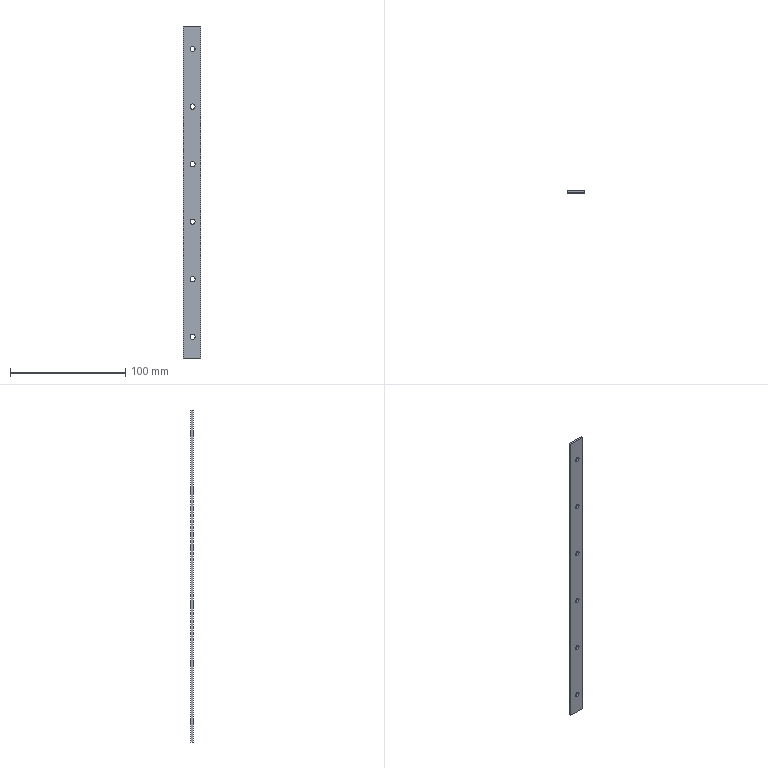Part | STEP file | Strip (L) | 1 solid | 18 faces | box 15 x 2 x 288.5 mm | volume 8464 mm3 | cylinder 12 | plane 6 | commonest cylinder face diameters 4.5 x12
STEP:
#1=CARTESIAN_POINT('',(0.,0.,0.));
#2=DIRECTION('',(0.,0.,1.));
#3=DIRECTION('',(1.,0.,0.));
#4=AXIS2_PLACEMENT_3D('',#1,#2,#3);
#5=CARTESIAN_POINT('',(8.,0.,16.25));
#6=VERTEX_POINT('',#5);
#7=CARTESIAN_POINT('',(8.,-2.,16.25));
#8=VERTEX_POINT('',#7);
#9=CARTESIAN_POINT('',(8.,-2.,16.25));
#10=DIRECTION('',(0.,-1.,0.));
#11=VECTOR('',#10,1.);
#12=LINE('',#9,#11);
#13=CARTESIAN_POINT('',(8.,-2.,18.5));
#14=DIRECTION('',(0.,-1.,0.));
#15=DIRECTION('',(0.,0.,-1.));
#16=AXIS2_PLACEMENT_3D('',#13,#14,#15);
#17=CYLINDRICAL_SURFACE('',#16,2.25);
#18=CARTESIAN_POINT('',(6.283,0.));
#19=DIRECTION('',(0.,1.));
#20=VECTOR('',#19,1.);
#21=LINE('',#18,#20);
#22=(GEOMETRIC_REPRESENTATION_CONTEXT(2)PARAMETRIC_REPRESENTATION_CONTEXT()REPRESENTATION_CONTEXT('',''));
#23=DEFINITIONAL_REPRESENTATION('',(#21),#22);
#24=PCURVE('',#17,#23);
#25=CARTESIAN_POINT('',(8.,-2.,18.5));
#26=DIRECTION('',(0.,-1.,0.));
#27=DIRECTION('',(0.,0.,-1.));
#28=AXIS2_PLACEMENT_3D('',#25,#26,#27);
#29=CYLINDRICAL_SURFACE('',#28,2.25);
#30=CARTESIAN_POINT('',(0.,0.));
#31=DIRECTION('',(0.,1.));
#32=VECTOR('',#31,1.);
#33=LINE('',#30,#32);
#34=(GEOMETRIC_REPRESENTATION_CONTEXT(2)PARAMETRIC_REPRESENTATION_CONTEXT()REPRESENTATION_CONTEXT('',''));
#35=DEFINITIONAL_REPRESENTATION('',(#33),#34);
#36=PCURVE('',#29,#35);
#37=SURFACE_CURVE('',#12,(#24,#36),.PCURVE_S1.);
#38=EDGE_CURVE('',#6,#8,#37,.T.);
#39=ORIENTED_EDGE('',*,*,#38,.T.);
#40=CARTESIAN_POINT('',(8.,-2.,20.75));
#41=VERTEX_POINT('',#40);
#42=CARTESIAN_POINT('',(8.,-2.,18.5));
#43=DIRECTION('',(0.,-1.,0.));
#44=DIRECTION('',(0.,0.,-1.));
#45=AXIS2_PLACEMENT_3D('',#42,#43,#44);
#46=CIRCLE('',#45,2.25);
#47=CARTESIAN_POINT('',(0.,0.));
#48=DIRECTION('',(1.,0.));
#49=VECTOR('',#48,1.);
#50=LINE('',#47,#49);
#51=(GEOMETRIC_REPRESENTATION_CONTEXT(2)PARAMETRIC_REPRESENTATION_CONTEXT()REPRESENTATION_CONTEXT('',''));
#52=DEFINITIONAL_REPRESENTATION('',(#50),#51);
#53=PCURVE('',#17,#52);
#54=CARTESIAN_POINT('',(0.,-2.,288.5));
#55=DIRECTION('',(0.,1.,0.));
#56=DIRECTION('',(0.,0.,1.));
#57=AXIS2_PLACEMENT_3D('',#54,#55,#56);
#58=PLANE('',#57);
#59=CARTESIAN_POINT('',(-272.25,8.));
#60=CARTESIAN_POINT('',(-272.25,11.897));
#61=CARTESIAN_POINT('',(-268.875,9.949));
#62=CARTESIAN_POINT('',(-265.5,8.));
#63=CARTESIAN_POINT('',(-268.875,6.051));
#64=CARTESIAN_POINT('',(-272.25,4.103));
#65=CARTESIAN_POINT('',(-272.25,8.));
#66=(BOUNDED_CURVE()B_SPLINE_CURVE(2,(#59,#60,#61,#62,#63,#64,#65),.UNSPECIFIED.,.T.,.F.)B_SPLINE_CURVE_WITH_KNOTS((1,2,2,2,2,1),(-2.094,0.,2.094,4.189,6.283,8.378),.UNSPECIFIED.)CURVE()GEOMETRIC_REPRESENTATION_ITEM()RATIONAL_B_SPLINE_CURVE((1.,0.5,1.,0.5,1.,0.5,1.))REPRESENTATION_ITEM(''));
#67=(GEOMETRIC_REPRESENTATION_CONTEXT(2)PARAMETRIC_REPRESENTATION_CONTEXT()REPRESENTATION_CONTEXT('',''));
#68=DEFINITIONAL_REPRESENTATION('',(#66),#67);
#69=PCURVE('',#58,#68);
#70=SURFACE_CURVE('',#46,(#53,#69),.PCURVE_S1.);
#71=EDGE_CURVE('',#41,#8,#70,.T.);
#72=ORIENTED_EDGE('',*,*,#71,.F.);
#73=CARTESIAN_POINT('',(8.,0.,20.75));
#74=VERTEX_POINT('',#73);
#75=CARTESIAN_POINT('',(8.,-2.,20.75));
#76=DIRECTION('',(0.,-1.,0.));
#77=VECTOR('',#76,1.);
#78=LINE('',#75,#77);
#79=CARTESIAN_POINT('',(3.142,0.));
#80=DIRECTION('',(0.,1.));
#81=VECTOR('',#80,1.);
#82=LINE('',#79,#81);
#83=(GEOMETRIC_REPRESENTATION_CONTEXT(2)PARAMETRIC_REPRESENTATION_CONTEXT()REPRESENTATION_CONTEXT('',''));
#84=DEFINITIONAL_REPRESENTATION('',(#82),#83);
#85=PCURVE('',#17,#84);
#86=CARTESIAN_POINT('',(3.142,0.));
#87=DIRECTION('',(0.,1.));
#88=VECTOR('',#87,1.);
#89=LINE('',#86,#88);
#90=(GEOMETRIC_REPRESENTATION_CONTEXT(2)PARAMETRIC_REPRESENTATION_CONTEXT()REPRESENTATION_CONTEXT('',''));
#91=DEFINITIONAL_REPRESENTATION('',(#89),#90);
#92=PCURVE('',#29,#91);
#93=SURFACE_CURVE('',#78,(#85,#92),.PCURVE_S1.);
#94=EDGE_CURVE('',#74,#41,#93,.T.);
#95=ORIENTED_EDGE('',*,*,#94,.F.);
#96=CARTESIAN_POINT('',(8.,0.,18.5));
#97=DIRECTION('',(0.,-1.,0.));
#98=DIRECTION('',(0.,0.,-1.));
#99=AXIS2_PLACEMENT_3D('',#96,#97,#98);
#100=CIRCLE('',#99,2.25);
#101=CARTESIAN_POINT('',(0.,-2.));
#102=DIRECTION('',(1.,0.));
#103=VECTOR('',#102,1.);
#104=LINE('',#101,#103);
#105=(GEOMETRIC_REPRESENTATION_CONTEXT(2)PARAMETRIC_REPRESENTATION_CONTEXT()REPRESENTATION_CONTEXT('',''));
#106=DEFINITIONAL_REPRESENTATION('',(#104),#105);
#107=PCURVE('',#17,#106);
#108=CARTESIAN_POINT('',(0.,0.,288.5));
#109=DIRECTION('',(0.,-1.,0.));
#110=DIRECTION('',(0.,0.,-1.));
#111=AXIS2_PLACEMENT_3D('',#108,#109,#110);
#112=PLANE('',#111);
#113=CARTESIAN_POINT('',(270.,8.));
#114=DIRECTION('',(1.,0.));
#115=AXIS2_PLACEMENT_2D('',#113,#114);
#116=CIRCLE('',#115,2.25);
#117=(GEOMETRIC_REPRESENTATION_CONTEXT(2)PARAMETRIC_REPRESENTATION_CONTEXT()REPRESENTATION_CONTEXT('',''));
#118=DEFINITIONAL_REPRESENTATION('',(#116),#117);
#119=PCURVE('',#112,#118);
#120=SURFACE_CURVE('',#100,(#107,#119),.PCURVE_S1.);
#121=EDGE_CURVE('',#74,#6,#120,.T.);
#122=ORIENTED_EDGE('',*,*,#121,.T.);
#123=EDGE_LOOP('',(#39,#72,#95,#122));
#124=FACE_BOUND('',#123,.F.);
#125=ADVANCED_FACE('',(#124),#17,.F.);
#126=CARTESIAN_POINT('',(8.,0.,66.25));
#127=VERTEX_POINT('',#126);
#128=CARTESIAN_POINT('',(8.,-2.,66.25));
#129=VERTEX_POINT('',#128);
#130=CARTESIAN_POINT('',(8.,-2.,66.25));
#131=DIRECTION('',(0.,-1.,0.));
#132=VECTOR('',#131,1.);
#133=LINE('',#130,#132);
#134=CARTESIAN_POINT('',(8.,-2.,68.5));
#135=DIRECTION('',(0.,-1.,0.));
#136=DIRECTION('',(0.,0.,-1.));
#137=AXIS2_PLACEMENT_3D('',#134,#135,#136);
#138=CYLINDRICAL_SURFACE('',#137,2.25);
#139=CARTESIAN_POINT('',(6.283,0.));
#140=DIRECTION('',(0.,1.));
#141=VECTOR('',#140,1.);
#142=LINE('',#139,#141);
#143=(GEOMETRIC_REPRESENTATION_CONTEXT(2)PARAMETRIC_REPRESENTATION_CONTEXT()REPRESENTATION_CONTEXT('',''));
#144=DEFINITIONAL_REPRESENTATION('',(#142),#143);
#145=PCURVE('',#138,#144);
#146=CARTESIAN_POINT('',(8.,-2.,68.5));
#147=DIRECTION('',(0.,-1.,0.));
#148=DIRECTION('',(0.,0.,-1.));
#149=AXIS2_PLACEMENT_3D('',#146,#147,#148);
#150=CYLINDRICAL_SURFACE('',#149,2.25);
#151=CARTESIAN_POINT('',(0.,0.));
#152=DIRECTION('',(0.,1.));
#153=VECTOR('',#152,1.);
#154=LINE('',#151,#153);
#155=(GEOMETRIC_REPRESENTATION_CONTEXT(2)PARAMETRIC_REPRESENTATION_CONTEXT()REPRESENTATION_CONTEXT('',''));
#156=DEFINITIONAL_REPRESENTATION('',(#154),#155);
#157=PCURVE('',#150,#156);
#158=SURFACE_CURVE('',#133,(#145,#157),.PCURVE_S1.);
#159=EDGE_CURVE('',#127,#129,#158,.T.);
#160=ORIENTED_EDGE('',*,*,#159,.T.);
#161=CARTESIAN_POINT('',(8.,-2.,70.75));
#162=VERTEX_POINT('',#161);
#163=CARTESIAN_POINT('',(8.,-2.,68.5));
#164=DIRECTION('',(0.,-1.,0.));
#165=DIRECTION('',(0.,0.,-1.));
#166=AXIS2_PLACEMENT_3D('',#163,#164,#165);
#167=CIRCLE('',#166,2.25);
#168=CARTESIAN_POINT('',(0.,0.));
#169=DIRECTION('',(1.,0.));
#170=VECTOR('',#169,1.);
#171=LINE('',#168,#170);
#172=(GEOMETRIC_REPRESENTATION_CONTEXT(2)PARAMETRIC_REPRESENTATION_CONTEXT()REPRESENTATION_CONTEXT('',''));
#173=DEFINITIONAL_REPRESENTATION('',(#171),#172);
#174=PCURVE('',#138,#173);
#175=CARTESIAN_POINT('',(-222.25,8.));
#176=CARTESIAN_POINT('',(-222.25,11.897));
#177=CARTESIAN_POINT('',(-218.875,9.949));
#178=CARTESIAN_POINT('',(-215.5,8.));
#179=CARTESIAN_POINT('',(-218.875,6.051));
#180=CARTESIAN_POINT('',(-222.25,4.103));
#181=CARTESIAN_POINT('',(-222.25,8.));
#182=(BOUNDED_CURVE()B_SPLINE_CURVE(2,(#175,#176,#177,#178,#179,#180,#181),.UNSPECIFIED.,.T.,.F.)B_SPLINE_CURVE_WITH_KNOTS((1,2,2,2,2,1),(-2.094,0.,2.094,4.189,6.283,8.378),.UNSPECIFIED.)CURVE()GEOMETRIC_REPRESENTATION_ITEM()RATIONAL_B_SPLINE_CURVE((1.,0.5,1.,0.5,1.,0.5,1.))REPRESENTATION_ITEM(''));
#183=(GEOMETRIC_REPRESENTATION_CONTEXT(2)PARAMETRIC_REPRESENTATION_CONTEXT()REPRESENTATION_CONTEXT('',''));
#184=DEFINITIONAL_REPRESENTATION('',(#182),#183);
#185=PCURVE('',#58,#184);
#186=SURFACE_CURVE('',#167,(#174,#185),.PCURVE_S1.);
#187=EDGE_CURVE('',#162,#129,#186,.T.);
#188=ORIENTED_EDGE('',*,*,#187,.F.);
#189=CARTESIAN_POINT('',(8.,0.,70.75));
#190=VERTEX_POINT('',#189);
#191=CARTESIAN_POINT('',(8.,-2.,70.75));
#192=DIRECTION('',(0.,-1.,0.));
#193=VECTOR('',#192,1.);
#194=LINE('',#191,#193);
#195=CARTESIAN_POINT('',(3.142,0.));
#196=DIRECTION('',(0.,1.));
#197=VECTOR('',#196,1.);
#198=LINE('',#195,#197);
#199=(GEOMETRIC_REPRESENTATION_CONTEXT(2)PARAMETRIC_REPRESENTATION_CONTEXT()REPRESENTATION_CONTEXT('',''));
#200=DEFINITIONAL_REPRESENTATION('',(#198),#199);
#201=PCURVE('',#138,#200);
#202=CARTESIAN_POINT('',(3.142,0.));
#203=DIRECTION('',(0.,1.));
#204=VECTOR('',#203,1.);
#205=LINE('',#202,#204);
#206=(GEOMETRIC_REPRESENTATION_CONTEXT(2)PARAMETRIC_REPRESENTATION_CONTEXT()REPRESENTATION_CONTEXT('',''));
#207=DEFINITIONAL_REPRESENTATION('',(#205),#206);
#208=PCURVE('',#150,#207);
#209=SURFACE_CURVE('',#194,(#201,#208),.PCURVE_S1.);
#210=EDGE_CURVE('',#190,#162,#209,.T.);
#211=ORIENTED_EDGE('',*,*,#210,.F.);
#212=CARTESIAN_POINT('',(8.,0.,68.5));
#213=DIRECTION('',(0.,-1.,0.));
#214=DIRECTION('',(0.,0.,-1.));
#215=AXIS2_PLACEMENT_3D('',#212,#213,#214);
#216=CIRCLE('',#215,2.25);
#217=CARTESIAN_POINT('',(0.,-2.));
#218=DIRECTION('',(1.,0.));
#219=VECTOR('',#218,1.);
#220=LINE('',#217,#219);
#221=(GEOMETRIC_REPRESENTATION_CONTEXT(2)PARAMETRIC_REPRESENTATION_CONTEXT()REPRESENTATION_CONTEXT('',''));
#222=DEFINITIONAL_REPRESENTATION('',(#220),#221);
#223=PCURVE('',#138,#222);
#224=CARTESIAN_POINT('',(220.,8.));
#225=DIRECTION('',(1.,0.));
#226=AXIS2_PLACEMENT_2D('',#224,#225);
#227=CIRCLE('',#226,2.25);
#228=(GEOMETRIC_REPRESENTATION_CONTEXT(2)PARAMETRIC_REPRESENTATION_CONTEXT()REPRESENTATION_CONTEXT('',''));
#229=DEFINITIONAL_REPRESENTATION('',(#227),#228);
#230=PCURVE('',#112,#229);
#231=SURFACE_CURVE('',#216,(#223,#230),.PCURVE_S1.);
#232=EDGE_CURVE('',#190,#127,#231,.T.);
#233=ORIENTED_EDGE('',*,*,#232,.T.);
#234=EDGE_LOOP('',(#160,#188,#211,#233));
#235=FACE_BOUND('',#234,.F.);
#236=ADVANCED_FACE('',(#235),#138,.F.);
#237=CARTESIAN_POINT('',(8.,0.,116.25));
#238=VERTEX_POINT('',#237);
#239=CARTESIAN_POINT('',(8.,-2.,116.25));
#240=VERTEX_POINT('',#239);
#241=CARTESIAN_POINT('',(8.,-2.,116.25));
#242=DIRECTION('',(0.,-1.,0.));
#243=VECTOR('',#242,1.);
#244=LINE('',#241,#243);
#245=CARTESIAN_POINT('',(8.,-2.,118.5));
#246=DIRECTION('',(0.,-1.,0.));
#247=DIRECTION('',(0.,0.,-1.));
#248=AXIS2_PLACEMENT_3D('',#245,#246,#247);
#249=CYLINDRICAL_SURFACE('',#248,2.25);
#250=CARTESIAN_POINT('',(6.283,0.));
#251=DIRECTION('',(0.,1.));
#252=VECTOR('',#251,1.);
#253=LINE('',#250,#252);
#254=(GEOMETRIC_REPRESENTATION_CONTEXT(2)PARAMETRIC_REPRESENTATION_CONTEXT()REPRESENTATION_CONTEXT('',''));
#255=DEFINITIONAL_REPRESENTATION('',(#253),#254);
#256=PCURVE('',#249,#255);
#257=CARTESIAN_POINT('',(8.,-2.,118.5));
#258=DIRECTION('',(0.,-1.,0.));
#259=DIRECTION('',(0.,0.,-1.));
#260=AXIS2_PLACEMENT_3D('',#257,#258,#259);
#261=CYLINDRICAL_SURFACE('',#260,2.25);
#262=CARTESIAN_POINT('',(0.,0.));
#263=DIRECTION('',(0.,1.));
#264=VECTOR('',#263,1.);
#265=LINE('',#262,#264);
#266=(GEOMETRIC_REPRESENTATION_CONTEXT(2)PARAMETRIC_REPRESENTATION_CONTEXT()REPRESENTATION_CONTEXT('',''));
#267=DEFINITIONAL_REPRESENTATION('',(#265),#266);
#268=PCURVE('',#261,#267);
#269=SURFACE_CURVE('',#244,(#256,#268),.PCURVE_S1.);
#270=EDGE_CURVE('',#238,#240,#269,.T.);
#271=ORIENTED_EDGE('',*,*,#270,.T.);
#272=CARTESIAN_POINT('',(8.,-2.,120.75));
#273=VERTEX_POINT('',#272);
#274=CARTESIAN_POINT('',(8.,-2.,118.5));
#275=DIRECTION('',(0.,-1.,0.));
#276=DIRECTION('',(0.,0.,-1.));
#277=AXIS2_PLACEMENT_3D('',#274,#275,#276);
#278=CIRCLE('',#277,2.25);
#279=CARTESIAN_POINT('',(0.,0.));
#280=DIRECTION('',(1.,0.));
#281=VECTOR('',#280,1.);
#282=LINE('',#279,#281);
#283=(GEOMETRIC_REPRESENTATION_CONTEXT(2)PARAMETRIC_REPRESENTATION_CONTEXT()REPRESENTATION_CONTEXT('',''));
#284=DEFINITIONAL_REPRESENTATION('',(#282),#283);
#285=PCURVE('',#249,#284);
#286=CARTESIAN_POINT('',(-172.25,8.));
#287=CARTESIAN_POINT('',(-172.25,11.897));
#288=CARTESIAN_POINT('',(-168.875,9.949));
#289=CARTESIAN_POINT('',(-165.5,8.));
#290=CARTESIAN_POINT('',(-168.875,6.051));
#291=CARTESIAN_POINT('',(-172.25,4.103));
#292=CARTESIAN_POINT('',(-172.25,8.));
#293=(BOUNDED_CURVE()B_SPLINE_CURVE(2,(#286,#287,#288,#289,#290,#291,#292),.UNSPECIFIED.,.T.,.F.)B_SPLINE_CURVE_WITH_KNOTS((1,2,2,2,2,1),(-2.094,0.,2.094,4.189,6.283,8.378),.UNSPECIFIED.)CURVE()GEOMETRIC_REPRESENTATION_ITEM()RATIONAL_B_SPLINE_CURVE((1.,0.5,1.,0.5,1.,0.5,1.))REPRESENTATION_ITEM(''));
#294=(GEOMETRIC_REPRESENTATION_CONTEXT(2)PARAMETRIC_REPRESENTATION_CONTEXT()REPRESENTATION_CONTEXT('',''));
#295=DEFINITIONAL_REPRESENTATION('',(#293),#294);
#296=PCURVE('',#58,#295);
#297=SURFACE_CURVE('',#278,(#285,#296),.PCURVE_S1.);
#298=EDGE_CURVE('',#273,#240,#297,.T.);
#299=ORIENTED_EDGE('',*,*,#298,.F.);
#300=CARTESIAN_POINT('',(8.,0.,120.75));
#301=VERTEX_POINT('',#300);
#302=CARTESIAN_POINT('',(8.,-2.,120.75));
#303=DIRECTION('',(0.,-1.,0.));
#304=VECTOR('',#303,1.);
#305=LINE('',#302,#304);
#306=CARTESIAN_POINT('',(3.142,0.));
#307=DIRECTION('',(0.,1.));
#308=VECTOR('',#307,1.);
#309=LINE('',#306,#308);
#310=(GEOMETRIC_REPRESENTATION_CONTEXT(2)PARAMETRIC_REPRESENTATION_CONTEXT()REPRESENTATION_CONTEXT('',''));
#311=DEFINITIONAL_REPRESENTATION('',(#309),#310);
#312=PCURVE('',#249,#311);
#313=CARTESIAN_POINT('',(3.142,0.));
#314=DIRECTION('',(0.,1.));
#315=VECTOR('',#314,1.);
#316=LINE('',#313,#315);
#317=(GEOMETRIC_REPRESENTATION_CONTEXT(2)PARAMETRIC_REPRESENTATION_CONTEXT()REPRESENTATION_CONTEXT('',''));
#318=DEFINITIONAL_REPRESENTATION('',(#316),#317);
#319=PCURVE('',#261,#318);
#320=SURFACE_CURVE('',#305,(#312,#319),.PCURVE_S1.);
#321=EDGE_CURVE('',#301,#273,#320,.T.);
#322=ORIENTED_EDGE('',*,*,#321,.F.);
#323=CARTESIAN_POINT('',(8.,0.,118.5));
#324=DIRECTION('',(0.,-1.,0.));
#325=DIRECTION('',(0.,0.,-1.));
#326=AXIS2_PLACEMENT_3D('',#323,#324,#325);
#327=CIRCLE('',#326,2.25);
#328=CARTESIAN_POINT('',(0.,-2.));
#329=DIRECTION('',(1.,0.));
#330=VECTOR('',#329,1.);
#331=LINE('',#328,#330);
#332=(GEOMETRIC_REPRESENTATION_CONTEXT(2)PARAMETRIC_REPRESENTATION_CONTEXT()REPRESENTATION_CONTEXT('',''));
#333=DEFINITIONAL_REPRESENTATION('',(#331),#332);
#334=PCURVE('',#249,#333);
#335=CARTESIAN_POINT('',(170.,8.));
#336=DIRECTION('',(1.,0.));
#337=AXIS2_PLACEMENT_2D('',#335,#336);
#338=CIRCLE('',#337,2.25);
#339=(GEOMETRIC_REPRESENTATION_CONTEXT(2)PARAMETRIC_REPRESENTATION_CONTEXT()REPRESENTATION_CONTEXT('',''));
#340=DEFINITIONAL_REPRESENTATION('',(#338),#339);
#341=PCURVE('',#112,#340);
#342=SURFACE_CURVE('',#327,(#334,#341),.PCURVE_S1.);
#343=EDGE_CURVE('',#301,#238,#342,.T.);
#344=ORIENTED_EDGE('',*,*,#343,.T.);
#345=EDGE_LOOP('',(#271,#299,#322,#344));
#346=FACE_BOUND('',#345,.F.);
#347=ADVANCED_FACE('',(#346),#249,.F.);
#348=CARTESIAN_POINT('',(8.,0.,166.25));
#349=VERTEX_POINT('',#348);
#350=CARTESIAN_POINT('',(8.,-2.,166.25));
#351=VERTEX_POINT('',#350);
#352=CARTESIAN_POINT('',(8.,-2.,166.25));
#353=DIRECTION('',(0.,-1.,0.));
#354=VECTOR('',#353,1.);
#355=LINE('',#352,#354);
#356=CARTESIAN_POINT('',(8.,-2.,168.5));
#357=DIRECTION('',(0.,-1.,0.));
#358=DIRECTION('',(0.,0.,-1.));
#359=AXIS2_PLACEMENT_3D('',#356,#357,#358);
#360=CYLINDRICAL_SURFACE('',#359,2.25);
#361=CARTESIAN_POINT('',(6.283,0.));
#362=DIRECTION('',(0.,1.));
#363=VECTOR('',#362,1.);
#364=LINE('',#361,#363);
#365=(GEOMETRIC_REPRESENTATION_CONTEXT(2)PARAMETRIC_REPRESENTATION_CONTEXT()REPRESENTATION_CONTEXT('',''));
#366=DEFINITIONAL_REPRESENTATION('',(#364),#365);
#367=PCURVE('',#360,#366);
#368=CARTESIAN_POINT('',(8.,-2.,168.5));
#369=DIRECTION('',(0.,-1.,0.));
#370=DIRECTION('',(0.,0.,-1.));
#371=AXIS2_PLACEMENT_3D('',#368,#369,#370);
#372=CYLINDRICAL_SURFACE('',#371,2.25);
#373=CARTESIAN_POINT('',(0.,0.));
#374=DIRECTION('',(0.,1.));
#375=VECTOR('',#374,1.);
#376=LINE('',#373,#375);
#377=(GEOMETRIC_REPRESENTATION_CONTEXT(2)PARAMETRIC_REPRESENTATION_CONTEXT()REPRESENTATION_CONTEXT('',''));
#378=DEFINITIONAL_REPRESENTATION('',(#376),#377);
#379=PCURVE('',#372,#378);
#380=SURFACE_CURVE('',#355,(#367,#379),.PCURVE_S1.);
#381=EDGE_CURVE('',#349,#351,#380,.T.);
#382=ORIENTED_EDGE('',*,*,#381,.T.);
#383=CARTESIAN_POINT('',(8.,-2.,170.75));
#384=VERTEX_POINT('',#383);
#385=CARTESIAN_POINT('',(8.,-2.,168.5));
#386=DIRECTION('',(0.,-1.,0.));
#387=DIRECTION('',(0.,0.,-1.));
#388=AXIS2_PLACEMENT_3D('',#385,#386,#387);
#389=CIRCLE('',#388,2.25);
#390=CARTESIAN_POINT('',(0.,0.));
#391=DIRECTION('',(1.,0.));
#392=VECTOR('',#391,1.);
#393=LINE('',#390,#392);
#394=(GEOMETRIC_REPRESENTATION_CONTEXT(2)PARAMETRIC_REPRESENTATION_CONTEXT()REPRESENTATION_CONTEXT('',''));
#395=DEFINITIONAL_REPRESENTATION('',(#393),#394);
#396=PCURVE('',#360,#395);
#397=CARTESIAN_POINT('',(-122.25,8.));
#398=CARTESIAN_POINT('',(-122.25,11.897));
#399=CARTESIAN_POINT('',(-118.875,9.949));
#400=CARTESIAN_POINT('',(-115.5,8.));
#401=CARTESIAN_POINT('',(-118.875,6.051));
#402=CARTESIAN_POINT('',(-122.25,4.103));
#403=CARTESIAN_POINT('',(-122.25,8.));
#404=(BOUNDED_CURVE()B_SPLINE_CURVE(2,(#397,#398,#399,#400,#401,#402,#403),.UNSPECIFIED.,.T.,.F.)B_SPLINE_CURVE_WITH_KNOTS((1,2,2,2,2,1),(-2.094,0.,2.094,4.189,6.283,8.378),.UNSPECIFIED.)CURVE()GEOMETRIC_REPRESENTATION_ITEM()RATIONAL_B_SPLINE_CURVE((1.,0.5,1.,0.5,1.,0.5,1.))REPRESENTATION_ITEM(''));
#405=(GEOMETRIC_REPRESENTATION_CONTEXT(2)PARAMETRIC_REPRESENTATION_CONTEXT()REPRESENTATION_CONTEXT('',''));
#406=DEFINITIONAL_REPRESENTATION('',(#404),#405);
#407=PCURVE('',#58,#406);
#408=SURFACE_CURVE('',#389,(#396,#407),.PCURVE_S1.);
#409=EDGE_CURVE('',#384,#351,#408,.T.);
#410=ORIENTED_EDGE('',*,*,#409,.F.);
#411=CARTESIAN_POINT('',(8.,0.,170.75));
#412=VERTEX_POINT('',#411);
#413=CARTESIAN_POINT('',(8.,-2.,170.75));
#414=DIRECTION('',(0.,-1.,0.));
#415=VECTOR('',#414,1.);
#416=LINE('',#413,#415);
#417=CARTESIAN_POINT('',(3.142,0.));
#418=DIRECTION('',(0.,1.));
#419=VECTOR('',#418,1.);
#420=LINE('',#417,#419);
#421=(GEOMETRIC_REPRESENTATION_CONTEXT(2)PARAMETRIC_REPRESENTATION_CONTEXT()REPRESENTATION_CONTEXT('',''));
#422=DEFINITIONAL_REPRESENTATION('',(#420),#421);
#423=PCURVE('',#360,#422);
#424=CARTESIAN_POINT('',(3.142,0.));
#425=DIRECTION('',(0.,1.));
#426=VECTOR('',#425,1.);
#427=LINE('',#424,#426);
#428=(GEOMETRIC_REPRESENTATION_CONTEXT(2)PARAMETRIC_REPRESENTATION_CONTEXT()REPRESENTATION_CONTEXT('',''));
#429=DEFINITIONAL_REPRESENTATION('',(#427),#428);
#430=PCURVE('',#372,#429);
#431=SURFACE_CURVE('',#416,(#423,#430),.PCURVE_S1.);
#432=EDGE_CURVE('',#412,#384,#431,.T.);
#433=ORIENTED_EDGE('',*,*,#432,.F.);
#434=CARTESIAN_POINT('',(8.,0.,168.5));
#435=DIRECTION('',(0.,-1.,0.));
#436=DIRECTION('',(0.,0.,-1.));
#437=AXIS2_PLACEMENT_3D('',#434,#435,#436);
#438=CIRCLE('',#437,2.25);
#439=CARTESIAN_POINT('',(0.,-2.));
#440=DIRECTION('',(1.,0.));
#441=VECTOR('',#440,1.);
#442=LINE('',#439,#441);
#443=(GEOMETRIC_REPRESENTATION_CONTEXT(2)PARAMETRIC_REPRESENTATION_CONTEXT()REPRESENTATION_CONTEXT('',''));
#444=DEFINITIONAL_REPRESENTATION('',(#442),#443);
#445=PCURVE('',#360,#444);
#446=CARTESIAN_POINT('',(120.,8.));
#447=DIRECTION('',(1.,0.));
#448=AXIS2_PLACEMENT_2D('',#446,#447);
#449=CIRCLE('',#448,2.25);
#450=(GEOMETRIC_REPRESENTATION_CONTEXT(2)PARAMETRIC_REPRESENTATION_CONTEXT()REPRESENTATION_CONTEXT('',''));
#451=DEFINITIONAL_REPRESENTATION('',(#449),#450);
#452=PCURVE('',#112,#451);
#453=SURFACE_CURVE('',#438,(#445,#452),.PCURVE_S1.);
#454=EDGE_CURVE('',#412,#349,#453,.T.);
#455=ORIENTED_EDGE('',*,*,#454,.T.);
#456=EDGE_LOOP('',(#382,#410,#433,#455));
#457=FACE_BOUND('',#456,.F.);
#458=ADVANCED_FACE('',(#457),#360,.F.);
#459=CARTESIAN_POINT('',(8.,0.,216.25));
#460=VERTEX_POINT('',#459);
#461=CARTESIAN_POINT('',(8.,-2.,216.25));
#462=VERTEX_POINT('',#461);
#463=CARTESIAN_POINT('',(8.,-2.,216.25));
#464=DIRECTION('',(0.,-1.,0.));
#465=VECTOR('',#464,1.);
#466=LINE('',#463,#465);
#467=CARTESIAN_POINT('',(8.,-2.,218.5));
#468=DIRECTION('',(0.,-1.,0.));
#469=DIRECTION('',(0.,0.,-1.));
#470=AXIS2_PLACEMENT_3D('',#467,#468,#469);
#471=CYLINDRICAL_SURFACE('',#470,2.25);
#472=CARTESIAN_POINT('',(6.283,0.));
#473=DIRECTION('',(0.,1.));
#474=VECTOR('',#473,1.);
#475=LINE('',#472,#474);
#476=(GEOMETRIC_REPRESENTATION_CONTEXT(2)PARAMETRIC_REPRESENTATION_CONTEXT()REPRESENTATION_CONTEXT('',''));
#477=DEFINITIONAL_REPRESENTATION('',(#475),#476);
#478=PCURVE('',#471,#477);
#479=CARTESIAN_POINT('',(8.,-2.,218.5));
#480=DIRECTION('',(0.,-1.,0.));
#481=DIRECTION('',(0.,0.,-1.));
#482=AXIS2_PLACEMENT_3D('',#479,#480,#481);
#483=CYLINDRICAL_SURFACE('',#482,2.25);
#484=CARTESIAN_POINT('',(0.,0.));
#485=DIRECTION('',(0.,1.));
#486=VECTOR('',#485,1.);
#487=LINE('',#484,#486);
#488=(GEOMETRIC_REPRESENTATION_CONTEXT(2)PARAMETRIC_REPRESENTATION_CONTEXT()REPRESENTATION_CONTEXT('',''));
#489=DEFINITIONAL_REPRESENTATION('',(#487),#488);
#490=PCURVE('',#483,#489);
#491=SURFACE_CURVE('',#466,(#478,#490),.PCURVE_S1.);
#492=EDGE_CURVE('',#460,#462,#491,.T.);
#493=ORIENTED_EDGE('',*,*,#492,.T.);
#494=CARTESIAN_POINT('',(8.,-2.,220.75));
#495=VERTEX_POINT('',#494);
#496=CARTESIAN_POINT('',(8.,-2.,218.5));
#497=DIRECTION('',(0.,-1.,0.));
#498=DIRECTION('',(0.,0.,-1.));
#499=AXIS2_PLACEMENT_3D('',#496,#497,#498);
#500=CIRCLE('',#499,2.25);
#501=CARTESIAN_POINT('',(0.,0.));
#502=DIRECTION('',(1.,0.));
#503=VECTOR('',#502,1.);
#504=LINE('',#501,#503);
#505=(GEOMETRIC_REPRESENTATION_CONTEXT(2)PARAMETRIC_REPRESENTATION_CONTEXT()REPRESENTATION_CONTEXT('',''));
#506=DEFINITIONAL_REPRESENTATION('',(#504),#505);
#507=PCURVE('',#471,#506);
#508=CARTESIAN_POINT('',(-72.25,8.));
#509=CARTESIAN_POINT('',(-72.25,11.897));
#510=CARTESIAN_POINT('',(-68.875,9.949));
#511=CARTESIAN_POINT('',(-65.5,8.));
#512=CARTESIAN_POINT('',(-68.875,6.051));
#513=CARTESIAN_POINT('',(-72.25,4.103));
#514=CARTESIAN_POINT('',(-72.25,8.));
#515=(BOUNDED_CURVE()B_SPLINE_CURVE(2,(#508,#509,#510,#511,#512,#513,#514),.UNSPECIFIED.,.T.,.F.)B_SPLINE_CURVE_WITH_KNOTS((1,2,2,2,2,1),(-2.094,0.,2.094,4.189,6.283,8.378),.UNSPECIFIED.)CURVE()GEOMETRIC_REPRESENTATION_ITEM()RATIONAL_B_SPLINE_CURVE((1.,0.5,1.,0.5,1.,0.5,1.))REPRESENTATION_ITEM(''));
#516=(GEOMETRIC_REPRESENTATION_CONTEXT(2)PARAMETRIC_REPRESENTATION_CONTEXT()REPRESENTATION_CONTEXT('',''));
#517=DEFINITIONAL_REPRESENTATION('',(#515),#516);
#518=PCURVE('',#58,#517);
#519=SURFACE_CURVE('',#500,(#507,#518),.PCURVE_S1.);
#520=EDGE_CURVE('',#495,#462,#519,.T.);
#521=ORIENTED_EDGE('',*,*,#520,.F.);
#522=CARTESIAN_POINT('',(8.,0.,220.75));
#523=VERTEX_POINT('',#522);
#524=CARTESIAN_POINT('',(8.,-2.,220.75));
#525=DIRECTION('',(0.,-1.,0.));
#526=VECTOR('',#525,1.);
#527=LINE('',#524,#526);
#528=CARTESIAN_POINT('',(3.142,0.));
#529=DIRECTION('',(0.,1.));
#530=VECTOR('',#529,1.);
#531=LINE('',#528,#530);
#532=(GEOMETRIC_REPRESENTATION_CONTEXT(2)PARAMETRIC_REPRESENTATION_CONTEXT()REPRESENTATION_CONTEXT('',''));
#533=DEFINITIONAL_REPRESENTATION('',(#531),#532);
#534=PCURVE('',#471,#533);
#535=CARTESIAN_POINT('',(3.142,0.));
#536=DIRECTION('',(0.,1.));
#537=VECTOR('',#536,1.);
#538=LINE('',#535,#537);
#539=(GEOMETRIC_REPRESENTATION_CONTEXT(2)PARAMETRIC_REPRESENTATION_CONTEXT()REPRESENTATION_CONTEXT('',''));
#540=DEFINITIONAL_REPRESENTATION('',(#538),#539);
#541=PCURVE('',#483,#540);
#542=SURFACE_CURVE('',#527,(#534,#541),.PCURVE_S1.);
#543=EDGE_CURVE('',#523,#495,#542,.T.);
#544=ORIENTED_EDGE('',*,*,#543,.F.);
#545=CARTESIAN_POINT('',(8.,0.,218.5));
#546=DIRECTION('',(0.,-1.,0.));
#547=DIRECTION('',(0.,0.,-1.));
#548=AXIS2_PLACEMENT_3D('',#545,#546,#547);
#549=CIRCLE('',#548,2.25);
#550=CARTESIAN_POINT('',(0.,-2.));
#551=DIRECTION('',(1.,0.));
#552=VECTOR('',#551,1.);
#553=LINE('',#550,#552);
#554=(GEOMETRIC_REPRESENTATION_CONTEXT(2)PARAMETRIC_REPRESENTATION_CONTEXT()REPRESENTATION_CONTEXT('',''));
#555=DEFINITIONAL_REPRESENTATION('',(#553),#554);
#556=PCURVE('',#471,#555);
#557=CARTESIAN_POINT('',(70.,8.));
#558=DIRECTION('',(1.,0.));
#559=AXIS2_PLACEMENT_2D('',#557,#558);
#560=CIRCLE('',#559,2.25);
#561=(GEOMETRIC_REPRESENTATION_CONTEXT(2)PARAMETRIC_REPRESENTATION_CONTEXT()REPRESENTATION_CONTEXT('',''));
#562=DEFINITIONAL_REPRESENTATION('',(#560),#561);
#563=PCURVE('',#112,#562);
#564=SURFACE_CURVE('',#549,(#556,#563),.PCURVE_S1.);
#565=EDGE_CURVE('',#523,#460,#564,.T.);
#566=ORIENTED_EDGE('',*,*,#565,.T.);
#567=EDGE_LOOP('',(#493,#521,#544,#566));
#568=FACE_BOUND('',#567,.F.);
#569=ADVANCED_FACE('',(#568),#471,.F.);
#570=CARTESIAN_POINT('',(8.,0.,266.25));
#571=VERTEX_POINT('',#570);
#572=CARTESIAN_POINT('',(8.,-2.,266.25));
#573=VERTEX_POINT('',#572);
#574=CARTESIAN_POINT('',(8.,-2.,266.25));
#575=DIRECTION('',(0.,-1.,0.));
#576=VECTOR('',#575,1.);
#577=LINE('',#574,#576);
#578=CARTESIAN_POINT('',(8.,-2.,268.5));
#579=DIRECTION('',(0.,-1.,0.));
#580=DIRECTION('',(0.,0.,-1.));
#581=AXIS2_PLACEMENT_3D('',#578,#579,#580);
#582=CYLINDRICAL_SURFACE('',#581,2.25);
#583=CARTESIAN_POINT('',(6.283,0.));
#584=DIRECTION('',(0.,1.));
#585=VECTOR('',#584,1.);
#586=LINE('',#583,#585);
#587=(GEOMETRIC_REPRESENTATION_CONTEXT(2)PARAMETRIC_REPRESENTATION_CONTEXT()REPRESENTATION_CONTEXT('',''));
#588=DEFINITIONAL_REPRESENTATION('',(#586),#587);
#589=PCURVE('',#582,#588);
#590=CARTESIAN_POINT('',(8.,-2.,268.5));
#591=DIRECTION('',(0.,-1.,0.));
#592=DIRECTION('',(0.,0.,-1.));
#593=AXIS2_PLACEMENT_3D('',#590,#591,#592);
#594=CYLINDRICAL_SURFACE('',#593,2.25);
#595=CARTESIAN_POINT('',(0.,0.));
#596=DIRECTION('',(0.,1.));
#597=VECTOR('',#596,1.);
#598=LINE('',#595,#597);
#599=(GEOMETRIC_REPRESENTATION_CONTEXT(2)PARAMETRIC_REPRESENTATION_CONTEXT()REPRESENTATION_CONTEXT('',''));
#600=DEFINITIONAL_REPRESENTATION('',(#598),#599);
#601=PCURVE('',#594,#600);
#602=SURFACE_CURVE('',#577,(#589,#601),.PCURVE_S1.);
#603=EDGE_CURVE('',#571,#573,#602,.T.);
#604=ORIENTED_EDGE('',*,*,#603,.T.);
#605=CARTESIAN_POINT('',(8.,-2.,270.75));
#606=VERTEX_POINT('',#605);
#607=CARTESIAN_POINT('',(8.,-2.,268.5));
#608=DIRECTION('',(0.,-1.,0.));
#609=DIRECTION('',(0.,0.,-1.));
#610=AXIS2_PLACEMENT_3D('',#607,#608,#609);
#611=CIRCLE('',#610,2.25);
#612=CARTESIAN_POINT('',(0.,0.));
#613=DIRECTION('',(1.,0.));
#614=VECTOR('',#613,1.);
#615=LINE('',#612,#614);
#616=(GEOMETRIC_REPRESENTATION_CONTEXT(2)PARAMETRIC_REPRESENTATION_CONTEXT()REPRESENTATION_CONTEXT('',''));
#617=DEFINITIONAL_REPRESENTATION('',(#615),#616);
#618=PCURVE('',#582,#617);
#619=CARTESIAN_POINT('',(-22.25,8.));
#620=CARTESIAN_POINT('',(-22.25,11.897));
#621=CARTESIAN_POINT('',(-18.875,9.949));
#622=CARTESIAN_POINT('',(-15.5,8.));
#623=CARTESIAN_POINT('',(-18.875,6.051));
#624=CARTESIAN_POINT('',(-22.25,4.103));
#625=CARTESIAN_POINT('',(-22.25,8.));
#626=(BOUNDED_CURVE()B_SPLINE_CURVE(2,(#619,#620,#621,#622,#623,#624,#625),.UNSPECIFIED.,.T.,.F.)B_SPLINE_CURVE_WITH_KNOTS((1,2,2,2,2,1),(-2.094,0.,2.094,4.189,6.283,8.378),.UNSPECIFIED.)CURVE()GEOMETRIC_REPRESENTATION_ITEM()RATIONAL_B_SPLINE_CURVE((1.,0.5,1.,0.5,1.,0.5,1.))REPRESENTATION_ITEM(''));
#627=(GEOMETRIC_REPRESENTATION_CONTEXT(2)PARAMETRIC_REPRESENTATION_CONTEXT()REPRESENTATION_CONTEXT('',''));
#628=DEFINITIONAL_REPRESENTATION('',(#626),#627);
#629=PCURVE('',#58,#628);
#630=SURFACE_CURVE('',#611,(#618,#629),.PCURVE_S1.);
#631=EDGE_CURVE('',#606,#573,#630,.T.);
#632=ORIENTED_EDGE('',*,*,#631,.F.);
#633=CARTESIAN_POINT('',(8.,0.,270.75));
#634=VERTEX_POINT('',#633);
#635=CARTESIAN_POINT('',(8.,-2.,270.75));
#636=DIRECTION('',(0.,-1.,0.));
#637=VECTOR('',#636,1.);
#638=LINE('',#635,#637);
#639=CARTESIAN_POINT('',(3.142,0.));
#640=DIRECTION('',(0.,1.));
#641=VECTOR('',#640,1.);
#642=LINE('',#639,#641);
#643=(GEOMETRIC_REPRESENTATION_CONTEXT(2)PARAMETRIC_REPRESENTATION_CONTEXT()REPRESENTATION_CONTEXT('',''));
#644=DEFINITIONAL_REPRESENTATION('',(#642),#643);
#645=PCURVE('',#582,#644);
#646=CARTESIAN_POINT('',(3.142,0.));
#647=DIRECTION('',(0.,1.));
#648=VECTOR('',#647,1.);
#649=LINE('',#646,#648);
#650=(GEOMETRIC_REPRESENTATION_CONTEXT(2)PARAMETRIC_REPRESENTATION_CONTEXT()REPRESENTATION_CONTEXT('',''));
#651=DEFINITIONAL_REPRESENTATION('',(#649),#650);
#652=PCURVE('',#594,#651);
#653=SURFACE_CURVE('',#638,(#645,#652),.PCURVE_S1.);
#654=EDGE_CURVE('',#634,#606,#653,.T.);
#655=ORIENTED_EDGE('',*,*,#654,.F.);
#656=CARTESIAN_POINT('',(8.,0.,268.5));
#657=DIRECTION('',(0.,-1.,0.));
#658=DIRECTION('',(0.,0.,-1.));
#659=AXIS2_PLACEMENT_3D('',#656,#657,#658);
#660=CIRCLE('',#659,2.25);
#661=CARTESIAN_POINT('',(0.,-2.));
#662=DIRECTION('',(1.,0.));
#663=VECTOR('',#662,1.);
#664=LINE('',#661,#663);
#665=(GEOMETRIC_REPRESENTATION_CONTEXT(2)PARAMETRIC_REPRESENTATION_CONTEXT()REPRESENTATION_CONTEXT('',''));
#666=DEFINITIONAL_REPRESENTATION('',(#664),#665);
#667=PCURVE('',#582,#666);
#668=CARTESIAN_POINT('',(20.,8.));
#669=DIRECTION('',(1.,0.));
#670=AXIS2_PLACEMENT_2D('',#668,#669);
#671=CIRCLE('',#670,2.25);
#672=(GEOMETRIC_REPRESENTATION_CONTEXT(2)PARAMETRIC_REPRESENTATION_CONTEXT()REPRESENTATION_CONTEXT('',''));
#673=DEFINITIONAL_REPRESENTATION('',(#671),#672);
#674=PCURVE('',#112,#673);
#675=SURFACE_CURVE('',#660,(#667,#674),.PCURVE_S1.);
#676=EDGE_CURVE('',#634,#571,#675,.T.);
#677=ORIENTED_EDGE('',*,*,#676,.T.);
#678=EDGE_LOOP('',(#604,#632,#655,#677));
#679=FACE_BOUND('',#678,.F.);
#680=ADVANCED_FACE('',(#679),#582,.F.);
#681=CARTESIAN_POINT('',(15.,-2.,288.5));
#682=VERTEX_POINT('',#681);
#683=CARTESIAN_POINT('',(15.,-2.,0.));
#684=VERTEX_POINT('',#683);
#685=CARTESIAN_POINT('',(15.,-2.,288.5));
#686=DIRECTION('',(0.,0.,-1.));
#687=VECTOR('',#686,1.);
#688=LINE('',#685,#687);
#689=CARTESIAN_POINT('',(0.,15.));
#690=DIRECTION('',(-1.,0.));
#691=VECTOR('',#690,1.);
#692=LINE('',#689,#691);
#693=(GEOMETRIC_REPRESENTATION_CONTEXT(2)PARAMETRIC_REPRESENTATION_CONTEXT()REPRESENTATION_CONTEXT('',''));
#694=DEFINITIONAL_REPRESENTATION('',(#692),#693);
#695=PCURVE('',#58,#694);
#696=CARTESIAN_POINT('',(15.,0.,288.5));
#697=DIRECTION('',(-1.,0.,0.));
#698=DIRECTION('',(0.,0.,1.));
#699=AXIS2_PLACEMENT_3D('',#696,#697,#698);
#700=PLANE('',#699);
#701=CARTESIAN_POINT('',(0.,-2.));
#702=DIRECTION('',(-1.,0.));
#703=VECTOR('',#702,1.);
#704=LINE('',#701,#703);
#705=(GEOMETRIC_REPRESENTATION_CONTEXT(2)PARAMETRIC_REPRESENTATION_CONTEXT()REPRESENTATION_CONTEXT('',''));
#706=DEFINITIONAL_REPRESENTATION('',(#704),#705);
#707=PCURVE('',#700,#706);
#708=SURFACE_CURVE('',#688,(#695,#707),.PCURVE_S1.);
#709=EDGE_CURVE('',#682,#684,#708,.T.);
#710=ORIENTED_EDGE('',*,*,#709,.F.);
#711=CARTESIAN_POINT('',(0.,-2.,288.5));
#712=VERTEX_POINT('',#711);
#713=CARTESIAN_POINT('',(0.,-2.,288.5));
#714=DIRECTION('',(1.,0.,0.));
#715=VECTOR('',#714,1.);
#716=LINE('',#713,#715);
#717=CARTESIAN_POINT('',(0.,0.));
#718=DIRECTION('',(0.,1.));
#719=VECTOR('',#718,1.);
#720=LINE('',#717,#719);
#721=(GEOMETRIC_REPRESENTATION_CONTEXT(2)PARAMETRIC_REPRESENTATION_CONTEXT()REPRESENTATION_CONTEXT('',''));
#722=DEFINITIONAL_REPRESENTATION('',(#720),#721);
#723=PCURVE('',#58,#722);
#724=CARTESIAN_POINT('',(0.,-2.,288.5));
#725=DIRECTION('',(0.,0.,1.));
#726=DIRECTION('',(1.,0.,0.));
#727=AXIS2_PLACEMENT_3D('',#724,#725,#726);
#728=PLANE('',#727);
#729=CARTESIAN_POINT('',(0.,0.));
#730=DIRECTION('',(1.,0.));
#731=VECTOR('',#730,1.);
#732=LINE('',#729,#731);
#733=(GEOMETRIC_REPRESENTATION_CONTEXT(2)PARAMETRIC_REPRESENTATION_CONTEXT()REPRESENTATION_CONTEXT('',''));
#734=DEFINITIONAL_REPRESENTATION('',(#732),#733);
#735=PCURVE('',#728,#734);
#736=SURFACE_CURVE('',#716,(#723,#735),.PCURVE_S1.);
#737=EDGE_CURVE('',#712,#682,#736,.T.);
#738=ORIENTED_EDGE('',*,*,#737,.F.);
#739=CARTESIAN_POINT('',(0.,-2.,0.));
#740=VERTEX_POINT('',#739);
#741=CARTESIAN_POINT('',(0.,-2.,288.5));
#742=DIRECTION('',(0.,0.,1.));
#743=VECTOR('',#742,1.);
#744=LINE('',#741,#743);
#745=CARTESIAN_POINT('',(0.,0.));
#746=DIRECTION('',(1.,0.));
#747=VECTOR('',#746,1.);
#748=LINE('',#745,#747);
#749=(GEOMETRIC_REPRESENTATION_CONTEXT(2)PARAMETRIC_REPRESENTATION_CONTEXT()REPRESENTATION_CONTEXT('',''));
#750=DEFINITIONAL_REPRESENTATION('',(#748),#749);
#751=PCURVE('',#58,#750);
#752=CARTESIAN_POINT('',(0.,0.,288.5));
#753=DIRECTION('',(1.,0.,0.));
#754=DIRECTION('',(0.,1.,0.));
#755=AXIS2_PLACEMENT_3D('',#752,#753,#754);
#756=PLANE('',#755);
#757=CARTESIAN_POINT('',(-2.,0.));
#758=DIRECTION('',(0.,1.));
#759=VECTOR('',#758,1.);
#760=LINE('',#757,#759);
#761=(GEOMETRIC_REPRESENTATION_CONTEXT(2)PARAMETRIC_REPRESENTATION_CONTEXT()REPRESENTATION_CONTEXT('',''));
#762=DEFINITIONAL_REPRESENTATION('',(#760),#761);
#763=PCURVE('',#756,#762);
#764=SURFACE_CURVE('',#744,(#751,#763),.PCURVE_S1.);
#765=EDGE_CURVE('',#740,#712,#764,.T.);
#766=ORIENTED_EDGE('',*,*,#765,.F.);
#767=CARTESIAN_POINT('',(0.,-2.,0.));
#768=DIRECTION('',(-1.,0.,0.));
#769=VECTOR('',#768,1.);
#770=LINE('',#767,#769);
#771=CARTESIAN_POINT('',(-288.5,0.));
#772=DIRECTION('',(0.,-1.));
#773=VECTOR('',#772,1.);
#774=LINE('',#771,#773);
#775=(GEOMETRIC_REPRESENTATION_CONTEXT(2)PARAMETRIC_REPRESENTATION_CONTEXT()REPRESENTATION_CONTEXT('',''));
#776=DEFINITIONAL_REPRESENTATION('',(#774),#775);
#777=PCURVE('',#58,#776);
#778=CARTESIAN_POINT('',(0.,-2.,0.));
#779=DIRECTION('',(0.,0.,1.));
#780=DIRECTION('',(1.,0.,0.));
#781=AXIS2_PLACEMENT_3D('',#778,#779,#780);
#782=PLANE('',#781);
#783=CARTESIAN_POINT('',(0.,0.));
#784=DIRECTION('',(-1.,0.));
#785=VECTOR('',#784,1.);
#786=LINE('',#783,#785);
#787=(GEOMETRIC_REPRESENTATION_CONTEXT(2)PARAMETRIC_REPRESENTATION_CONTEXT()REPRESENTATION_CONTEXT('',''));
#788=DEFINITIONAL_REPRESENTATION('',(#786),#787);
#789=PCURVE('',#782,#788);
#790=SURFACE_CURVE('',#770,(#777,#789),.PCURVE_S1.);
#791=EDGE_CURVE('',#684,#740,#790,.T.);
#792=ORIENTED_EDGE('',*,*,#791,.F.);
#793=EDGE_LOOP('',(#710,#738,#766,#792));
#794=FACE_BOUND('',#793,.T.);
#795=CARTESIAN_POINT('',(8.,-2.,18.5));
#796=DIRECTION('',(0.,-1.,0.));
#797=DIRECTION('',(0.,0.,-1.));
#798=AXIS2_PLACEMENT_3D('',#795,#796,#797);
#799=CIRCLE('',#798,2.25);
#800=CARTESIAN_POINT('',(-272.25,8.));
#801=CARTESIAN_POINT('',(-272.25,11.897));
#802=CARTESIAN_POINT('',(-268.875,9.949));
#803=CARTESIAN_POINT('',(-265.5,8.));
#804=CARTESIAN_POINT('',(-268.875,6.051));
#805=CARTESIAN_POINT('',(-272.25,4.103));
#806=CARTESIAN_POINT('',(-272.25,8.));
#807=(BOUNDED_CURVE()B_SPLINE_CURVE(2,(#800,#801,#802,#803,#804,#805,#806),.UNSPECIFIED.,.T.,.F.)B_SPLINE_CURVE_WITH_KNOTS((1,2,2,2,2,1),(-2.094,0.,2.094,4.189,6.283,8.378),.UNSPECIFIED.)CURVE()GEOMETRIC_REPRESENTATION_ITEM()RATIONAL_B_SPLINE_CURVE((1.,0.5,1.,0.5,1.,0.5,1.))REPRESENTATION_ITEM(''));
#808=(GEOMETRIC_REPRESENTATION_CONTEXT(2)PARAMETRIC_REPRESENTATION_CONTEXT()REPRESENTATION_CONTEXT('',''));
#809=DEFINITIONAL_REPRESENTATION('',(#807),#808);
#810=PCURVE('',#58,#809);
#811=CARTESIAN_POINT('',(0.,0.));
#812=DIRECTION('',(1.,0.));
#813=VECTOR('',#812,1.);
#814=LINE('',#811,#813);
#815=(GEOMETRIC_REPRESENTATION_CONTEXT(2)PARAMETRIC_REPRESENTATION_CONTEXT()REPRESENTATION_CONTEXT('',''));
#816=DEFINITIONAL_REPRESENTATION('',(#814),#815);
#817=PCURVE('',#29,#816);
#818=SURFACE_CURVE('',#799,(#810,#817),.PCURVE_S1.);
#819=EDGE_CURVE('',#8,#41,#818,.T.);
#820=ORIENTED_EDGE('',*,*,#819,.F.);
#821=ORIENTED_EDGE('',*,*,#71,.F.);
#822=EDGE_LOOP('',(#820,#821));
#823=FACE_BOUND('',#822,.T.);
#824=CARTESIAN_POINT('',(8.,-2.,68.5));
#825=DIRECTION('',(0.,-1.,0.));
#826=DIRECTION('',(0.,0.,-1.));
#827=AXIS2_PLACEMENT_3D('',#824,#825,#826);
#828=CIRCLE('',#827,2.25);
#829=CARTESIAN_POINT('',(-222.25,8.));
#830=CARTESIAN_POINT('',(-222.25,11.897));
#831=CARTESIAN_POINT('',(-218.875,9.949));
#832=CARTESIAN_POINT('',(-215.5,8.));
#833=CARTESIAN_POINT('',(-218.875,6.051));
#834=CARTESIAN_POINT('',(-222.25,4.103));
#835=CARTESIAN_POINT('',(-222.25,8.));
#836=(BOUNDED_CURVE()B_SPLINE_CURVE(2,(#829,#830,#831,#832,#833,#834,#835),.UNSPECIFIED.,.T.,.F.)B_SPLINE_CURVE_WITH_KNOTS((1,2,2,2,2,1),(-2.094,0.,2.094,4.189,6.283,8.378),.UNSPECIFIED.)CURVE()GEOMETRIC_REPRESENTATION_ITEM()RATIONAL_B_SPLINE_CURVE((1.,0.5,1.,0.5,1.,0.5,1.))REPRESENTATION_ITEM(''));
#837=(GEOMETRIC_REPRESENTATION_CONTEXT(2)PARAMETRIC_REPRESENTATION_CONTEXT()REPRESENTATION_CONTEXT('',''));
#838=DEFINITIONAL_REPRESENTATION('',(#836),#837);
#839=PCURVE('',#58,#838);
#840=CARTESIAN_POINT('',(0.,0.));
#841=DIRECTION('',(1.,0.));
#842=VECTOR('',#841,1.);
#843=LINE('',#840,#842);
#844=(GEOMETRIC_REPRESENTATION_CONTEXT(2)PARAMETRIC_REPRESENTATION_CONTEXT()REPRESENTATION_CONTEXT('',''));
#845=DEFINITIONAL_REPRESENTATION('',(#843),#844);
#846=PCURVE('',#150,#845);
#847=SURFACE_CURVE('',#828,(#839,#846),.PCURVE_S1.);
#848=EDGE_CURVE('',#129,#162,#847,.T.);
#849=ORIENTED_EDGE('',*,*,#848,.F.);
#850=ORIENTED_EDGE('',*,*,#187,.F.);
#851=EDGE_LOOP('',(#849,#850));
#852=FACE_BOUND('',#851,.T.);
#853=CARTESIAN_POINT('',(8.,-2.,118.5));
#854=DIRECTION('',(0.,-1.,0.));
#855=DIRECTION('',(0.,0.,-1.));
#856=AXIS2_PLACEMENT_3D('',#853,#854,#855);
#857=CIRCLE('',#856,2.25);
#858=CARTESIAN_POINT('',(-172.25,8.));
#859=CARTESIAN_POINT('',(-172.25,11.897));
#860=CARTESIAN_POINT('',(-168.875,9.949));
#861=CARTESIAN_POINT('',(-165.5,8.));
#862=CARTESIAN_POINT('',(-168.875,6.051));
#863=CARTESIAN_POINT('',(-172.25,4.103));
#864=CARTESIAN_POINT('',(-172.25,8.));
#865=(BOUNDED_CURVE()B_SPLINE_CURVE(2,(#858,#859,#860,#861,#862,#863,#864),.UNSPECIFIED.,.T.,.F.)B_SPLINE_CURVE_WITH_KNOTS((1,2,2,2,2,1),(-2.094,0.,2.094,4.189,6.283,8.378),.UNSPECIFIED.)CURVE()GEOMETRIC_REPRESENTATION_ITEM()RATIONAL_B_SPLINE_CURVE((1.,0.5,1.,0.5,1.,0.5,1.))REPRESENTATION_ITEM(''));
#866=(GEOMETRIC_REPRESENTATION_CONTEXT(2)PARAMETRIC_REPRESENTATION_CONTEXT()REPRESENTATION_CONTEXT('',''));
#867=DEFINITIONAL_REPRESENTATION('',(#865),#866);
#868=PCURVE('',#58,#867);
#869=CARTESIAN_POINT('',(0.,0.));
#870=DIRECTION('',(1.,0.));
#871=VECTOR('',#870,1.);
#872=LINE('',#869,#871);
#873=(GEOMETRIC_REPRESENTATION_CONTEXT(2)PARAMETRIC_REPRESENTATION_CONTEXT()REPRESENTATION_CONTEXT('',''));
#874=DEFINITIONAL_REPRESENTATION('',(#872),#873);
#875=PCURVE('',#261,#874);
#876=SURFACE_CURVE('',#857,(#868,#875),.PCURVE_S1.);
#877=EDGE_CURVE('',#240,#273,#876,.T.);
#878=ORIENTED_EDGE('',*,*,#877,.F.);
#879=ORIENTED_EDGE('',*,*,#298,.F.);
#880=EDGE_LOOP('',(#878,#879));
#881=FACE_BOUND('',#880,.T.);
#882=CARTESIAN_POINT('',(8.,-2.,168.5));
#883=DIRECTION('',(0.,-1.,0.));
#884=DIRECTION('',(0.,0.,-1.));
#885=AXIS2_PLACEMENT_3D('',#882,#883,#884);
#886=CIRCLE('',#885,2.25);
#887=CARTESIAN_POINT('',(-122.25,8.));
#888=CARTESIAN_POINT('',(-122.25,11.897));
#889=CARTESIAN_POINT('',(-118.875,9.949));
#890=CARTESIAN_POINT('',(-115.5,8.));
#891=CARTESIAN_POINT('',(-118.875,6.051));
#892=CARTESIAN_POINT('',(-122.25,4.103));
#893=CARTESIAN_POINT('',(-122.25,8.));
#894=(BOUNDED_CURVE()B_SPLINE_CURVE(2,(#887,#888,#889,#890,#891,#892,#893),.UNSPECIFIED.,.T.,.F.)B_SPLINE_CURVE_WITH_KNOTS((1,2,2,2,2,1),(-2.094,0.,2.094,4.189,6.283,8.378),.UNSPECIFIED.)CURVE()GEOMETRIC_REPRESENTATION_ITEM()RATIONAL_B_SPLINE_CURVE((1.,0.5,1.,0.5,1.,0.5,1.))REPRESENTATION_ITEM(''));
#895=(GEOMETRIC_REPRESENTATION_CONTEXT(2)PARAMETRIC_REPRESENTATION_CONTEXT()REPRESENTATION_CONTEXT('',''));
#896=DEFINITIONAL_REPRESENTATION('',(#894),#895);
#897=PCURVE('',#58,#896);
#898=CARTESIAN_POINT('',(0.,0.));
#899=DIRECTION('',(1.,0.));
#900=VECTOR('',#899,1.);
#901=LINE('',#898,#900);
#902=(GEOMETRIC_REPRESENTATION_CONTEXT(2)PARAMETRIC_REPRESENTATION_CONTEXT()REPRESENTATION_CONTEXT('',''));
#903=DEFINITIONAL_REPRESENTATION('',(#901),#902);
#904=PCURVE('',#372,#903);
#905=SURFACE_CURVE('',#886,(#897,#904),.PCURVE_S1.);
#906=EDGE_CURVE('',#351,#384,#905,.T.);
#907=ORIENTED_EDGE('',*,*,#906,.F.);
#908=ORIENTED_EDGE('',*,*,#409,.F.);
#909=EDGE_LOOP('',(#907,#908));
#910=FACE_BOUND('',#909,.T.);
#911=CARTESIAN_POINT('',(8.,-2.,218.5));
#912=DIRECTION('',(0.,-1.,0.));
#913=DIRECTION('',(0.,0.,-1.));
#914=AXIS2_PLACEMENT_3D('',#911,#912,#913);
#915=CIRCLE('',#914,2.25);
#916=CARTESIAN_POINT('',(-72.25,8.));
#917=CARTESIAN_POINT('',(-72.25,11.897));
#918=CARTESIAN_POINT('',(-68.875,9.949));
#919=CARTESIAN_POINT('',(-65.5,8.));
#920=CARTESIAN_POINT('',(-68.875,6.051));
#921=CARTESIAN_POINT('',(-72.25,4.103));
#922=CARTESIAN_POINT('',(-72.25,8.));
#923=(BOUNDED_CURVE()B_SPLINE_CURVE(2,(#916,#917,#918,#919,#920,#921,#922),.UNSPECIFIED.,.T.,.F.)B_SPLINE_CURVE_WITH_KNOTS((1,2,2,2,2,1),(-2.094,0.,2.094,4.189,6.283,8.378),.UNSPECIFIED.)CURVE()GEOMETRIC_REPRESENTATION_ITEM()RATIONAL_B_SPLINE_CURVE((1.,0.5,1.,0.5,1.,0.5,1.))REPRESENTATION_ITEM(''));
#924=(GEOMETRIC_REPRESENTATION_CONTEXT(2)PARAMETRIC_REPRESENTATION_CONTEXT()REPRESENTATION_CONTEXT('',''));
#925=DEFINITIONAL_REPRESENTATION('',(#923),#924);
#926=PCURVE('',#58,#925);
#927=CARTESIAN_POINT('',(0.,0.));
#928=DIRECTION('',(1.,0.));
#929=VECTOR('',#928,1.);
#930=LINE('',#927,#929);
#931=(GEOMETRIC_REPRESENTATION_CONTEXT(2)PARAMETRIC_REPRESENTATION_CONTEXT()REPRESENTATION_CONTEXT('',''));
#932=DEFINITIONAL_REPRESENTATION('',(#930),#931);
#933=PCURVE('',#483,#932);
#934=SURFACE_CURVE('',#915,(#926,#933),.PCURVE_S1.);
#935=EDGE_CURVE('',#462,#495,#934,.T.);
#936=ORIENTED_EDGE('',*,*,#935,.F.);
#937=ORIENTED_EDGE('',*,*,#520,.F.);
#938=EDGE_LOOP('',(#936,#937));
#939=FACE_BOUND('',#938,.T.);
#940=CARTESIAN_POINT('',(8.,-2.,268.5));
#941=DIRECTION('',(0.,-1.,0.));
#942=DIRECTION('',(0.,0.,-1.));
#943=AXIS2_PLACEMENT_3D('',#940,#941,#942);
#944=CIRCLE('',#943,2.25);
#945=CARTESIAN_POINT('',(-22.25,8.));
#946=CARTESIAN_POINT('',(-22.25,11.897));
#947=CARTESIAN_POINT('',(-18.875,9.949));
#948=CARTESIAN_POINT('',(-15.5,8.));
#949=CARTESIAN_POINT('',(-18.875,6.051));
#950=CARTESIAN_POINT('',(-22.25,4.103));
#951=CARTESIAN_POINT('',(-22.25,8.));
#952=(BOUNDED_CURVE()B_SPLINE_CURVE(2,(#945,#946,#947,#948,#949,#950,#951),.UNSPECIFIED.,.T.,.F.)B_SPLINE_CURVE_WITH_KNOTS((1,2,2,2,2,1),(-2.094,0.,2.094,4.189,6.283,8.378),.UNSPECIFIED.)CURVE()GEOMETRIC_REPRESENTATION_ITEM()RATIONAL_B_SPLINE_CURVE((1.,0.5,1.,0.5,1.,0.5,1.))REPRESENTATION_ITEM(''));
#953=(GEOMETRIC_REPRESENTATION_CONTEXT(2)PARAMETRIC_REPRESENTATION_CONTEXT()REPRESENTATION_CONTEXT('',''));
#954=DEFINITIONAL_REPRESENTATION('',(#952),#953);
#955=PCURVE('',#58,#954);
#956=CARTESIAN_POINT('',(0.,0.));
#957=DIRECTION('',(1.,0.));
#958=VECTOR('',#957,1.);
#959=LINE('',#956,#958);
#960=(GEOMETRIC_REPRESENTATION_CONTEXT(2)PARAMETRIC_REPRESENTATION_CONTEXT()REPRESENTATION_CONTEXT('',''));
#961=DEFINITIONAL_REPRESENTATION('',(#959),#960);
#962=PCURVE('',#594,#961);
#963=SURFACE_CURVE('',#944,(#955,#962),.PCURVE_S1.);
#964=EDGE_CURVE('',#573,#606,#963,.T.);
#965=ORIENTED_EDGE('',*,*,#964,.F.);
#966=ORIENTED_EDGE('',*,*,#631,.F.);
#967=EDGE_LOOP('',(#965,#966));
#968=FACE_BOUND('',#967,.T.);
#969=ADVANCED_FACE('',(#794,#823,#852,#881,#910,#939,#968),#58,.F.);
#970=CARTESIAN_POINT('',(15.,0.,0.));
#971=VERTEX_POINT('',#970);
#972=CARTESIAN_POINT('',(0.,0.,0.));
#973=VERTEX_POINT('',#972);
#974=CARTESIAN_POINT('',(0.,0.,0.));
#975=DIRECTION('',(-1.,0.,0.));
#976=VECTOR('',#975,1.);
#977=LINE('',#974,#976);
#978=CARTESIAN_POINT('',(0.,2.));
#979=DIRECTION('',(-1.,0.));
#980=VECTOR('',#979,1.);
#981=LINE('',#978,#980);
#982=(GEOMETRIC_REPRESENTATION_CONTEXT(2)PARAMETRIC_REPRESENTATION_CONTEXT()REPRESENTATION_CONTEXT('',''));
#983=DEFINITIONAL_REPRESENTATION('',(#981),#982);
#984=PCURVE('',#782,#983);
#985=CARTESIAN_POINT('',(288.5,0.));
#986=DIRECTION('',(0.,-1.));
#987=VECTOR('',#986,1.);
#988=LINE('',#985,#987);
#989=(GEOMETRIC_REPRESENTATION_CONTEXT(2)PARAMETRIC_REPRESENTATION_CONTEXT()REPRESENTATION_CONTEXT('',''));
#990=DEFINITIONAL_REPRESENTATION('',(#988),#989);
#991=PCURVE('',#112,#990);
#992=SURFACE_CURVE('',#977,(#984,#991),.PCURVE_S1.);
#993=EDGE_CURVE('',#971,#973,#992,.T.);
#994=ORIENTED_EDGE('',*,*,#993,.F.);
#995=CARTESIAN_POINT('',(15.,-2.,0.));
#996=DIRECTION('',(0.,1.,0.));
#997=VECTOR('',#996,1.);
#998=LINE('',#995,#997);
#999=CARTESIAN_POINT('',(15.,0.));
#1000=DIRECTION('',(0.,1.));
#1001=VECTOR('',#1000,1.);
#1002=LINE('',#999,#1001);
#1003=(GEOMETRIC_REPRESENTATION_CONTEXT(2)PARAMETRIC_REPRESENTATION_CONTEXT()REPRESENTATION_CONTEXT('',''));
#1004=DEFINITIONAL_REPRESENTATION('',(#1002),#1003);
#1005=PCURVE('',#782,#1004);
#1006=CARTESIAN_POINT('',(-288.5,-2.));
#1007=DIRECTION('',(0.,1.));
#1008=VECTOR('',#1007,1.);
#1009=LINE('',#1006,#1008);
#1010=(GEOMETRIC_REPRESENTATION_CONTEXT(2)PARAMETRIC_REPRESENTATION_CONTEXT()REPRESENTATION_CONTEXT('',''));
#1011=DEFINITIONAL_REPRESENTATION('',(#1009),#1010);
#1012=PCURVE('',#700,#1011);
#1013=SURFACE_CURVE('',#998,(#1005,#1012),.PCURVE_S1.);
#1014=EDGE_CURVE('',#684,#971,#1013,.T.);
#1015=ORIENTED_EDGE('',*,*,#1014,.F.);
#1016=ORIENTED_EDGE('',*,*,#791,.T.);
#1017=CARTESIAN_POINT('',(0.,-2.,0.));
#1018=DIRECTION('',(0.,-1.,0.));
#1019=VECTOR('',#1018,1.);
#1020=LINE('',#1017,#1019);
#1021=CARTESIAN_POINT('',(0.,0.));
#1022=DIRECTION('',(0.,-1.));
#1023=VECTOR('',#1022,1.);
#1024=LINE('',#1021,#1023);
#1025=(GEOMETRIC_REPRESENTATION_CONTEXT(2)PARAMETRIC_REPRESENTATION_CONTEXT()REPRESENTATION_CONTEXT('',''));
#1026=DEFINITIONAL_REPRESENTATION('',(#1024),#1025);
#1027=PCURVE('',#782,#1026);
#1028=CARTESIAN_POINT('',(-2.,-288.5));
#1029=DIRECTION('',(-1.,0.));
#1030=VECTOR('',#1029,1.);
#1031=LINE('',#1028,#1030);
#1032=(GEOMETRIC_REPRESENTATION_CONTEXT(2)PARAMETRIC_REPRESENTATION_CONTEXT()REPRESENTATION_CONTEXT('',''));
#1033=DEFINITIONAL_REPRESENTATION('',(#1031),#1032);
#1034=PCURVE('',#756,#1033);
#1035=SURFACE_CURVE('',#1020,(#1027,#1034),.PCURVE_S1.);
#1036=EDGE_CURVE('',#973,#740,#1035,.T.);
#1037=ORIENTED_EDGE('',*,*,#1036,.F.);
#1038=EDGE_LOOP('',(#994,#1015,#1016,#1037));
#1039=FACE_BOUND('',#1038,.T.);
#1040=ADVANCED_FACE('',(#1039),#782,.F.);
#1041=CARTESIAN_POINT('',(15.,0.,288.5));
#1042=VERTEX_POINT('',#1041);
#1043=CARTESIAN_POINT('',(15.,0.,288.5));
#1044=DIRECTION('',(0.,0.,-1.));
#1045=VECTOR('',#1044,1.);
#1046=LINE('',#1043,#1045);
#1047=CARTESIAN_POINT('',(0.,0.));
#1048=DIRECTION('',(-1.,0.));
#1049=VECTOR('',#1048,1.);
#1050=LINE('',#1047,#1049);
#1051=(GEOMETRIC_REPRESENTATION_CONTEXT(2)PARAMETRIC_REPRESENTATION_CONTEXT()REPRESENTATION_CONTEXT('',''));
#1052=DEFINITIONAL_REPRESENTATION('',(#1050),#1051);
#1053=PCURVE('',#700,#1052);
#1054=CARTESIAN_POINT('',(0.,15.));
#1055=DIRECTION('',(1.,0.));
#1056=VECTOR('',#1055,1.);
#1057=LINE('',#1054,#1056);
#1058=(GEOMETRIC_REPRESENTATION_CONTEXT(2)PARAMETRIC_REPRESENTATION_CONTEXT()REPRESENTATION_CONTEXT('',''));
#1059=DEFINITIONAL_REPRESENTATION('',(#1057),#1058);
#1060=PCURVE('',#112,#1059);
#1061=SURFACE_CURVE('',#1046,(#1053,#1060),.PCURVE_S1.);
#1062=EDGE_CURVE('',#1042,#971,#1061,.T.);
#1063=ORIENTED_EDGE('',*,*,#1062,.F.);
#1064=CARTESIAN_POINT('',(15.,0.,288.5));
#1065=DIRECTION('',(0.,1.,0.));
#1066=VECTOR('',#1065,1.);
#1067=LINE('',#1064,#1066);
#1068=CARTESIAN_POINT('',(0.,0.));
#1069=DIRECTION('',(0.,1.));
#1070=VECTOR('',#1069,1.);
#1071=LINE('',#1068,#1070);
#1072=(GEOMETRIC_REPRESENTATION_CONTEXT(2)PARAMETRIC_REPRESENTATION_CONTEXT()REPRESENTATION_CONTEXT('',''));
#1073=DEFINITIONAL_REPRESENTATION('',(#1071),#1072);
#1074=PCURVE('',#700,#1073);
#1075=CARTESIAN_POINT('',(15.,2.));
#1076=DIRECTION('',(0.,1.));
#1077=VECTOR('',#1076,1.);
#1078=LINE('',#1075,#1077);
#1079=(GEOMETRIC_REPRESENTATION_CONTEXT(2)PARAMETRIC_REPRESENTATION_CONTEXT()REPRESENTATION_CONTEXT('',''));
#1080=DEFINITIONAL_REPRESENTATION('',(#1078),#1079);
#1081=PCURVE('',#728,#1080);
#1082=SURFACE_CURVE('',#1067,(#1074,#1081),.PCURVE_S1.);
#1083=EDGE_CURVE('',#682,#1042,#1082,.T.);
#1084=ORIENTED_EDGE('',*,*,#1083,.F.);
#1085=ORIENTED_EDGE('',*,*,#709,.T.);
#1086=ORIENTED_EDGE('',*,*,#1014,.T.);
#1087=EDGE_LOOP('',(#1063,#1084,#1085,#1086));
#1088=FACE_BOUND('',#1087,.T.);
#1089=ADVANCED_FACE('',(#1088),#700,.F.);
#1090=ORIENTED_EDGE('',*,*,#1083,.T.);
#1091=CARTESIAN_POINT('',(0.,0.,288.5));
#1092=VERTEX_POINT('',#1091);
#1093=CARTESIAN_POINT('',(0.,0.,288.5));
#1094=DIRECTION('',(-1.,0.,0.));
#1095=VECTOR('',#1094,1.);
#1096=LINE('',#1093,#1095);
#1097=CARTESIAN_POINT('',(0.,2.));
#1098=DIRECTION('',(-1.,0.));
#1099=VECTOR('',#1098,1.);
#1100=LINE('',#1097,#1099);
#1101=(GEOMETRIC_REPRESENTATION_CONTEXT(2)PARAMETRIC_REPRESENTATION_CONTEXT()REPRESENTATION_CONTEXT('',''));
#1102=DEFINITIONAL_REPRESENTATION('',(#1100),#1101);
#1103=PCURVE('',#728,#1102);
#1104=CARTESIAN_POINT('',(0.,0.));
#1105=DIRECTION('',(0.,-1.));
#1106=VECTOR('',#1105,1.);
#1107=LINE('',#1104,#1106);
#1108=(GEOMETRIC_REPRESENTATION_CONTEXT(2)PARAMETRIC_REPRESENTATION_CONTEXT()REPRESENTATION_CONTEXT('',''));
#1109=DEFINITIONAL_REPRESENTATION('',(#1107),#1108);
#1110=PCURVE('',#112,#1109);
#1111=SURFACE_CURVE('',#1096,(#1103,#1110),.PCURVE_S1.);
#1112=EDGE_CURVE('',#1042,#1092,#1111,.T.);
#1113=ORIENTED_EDGE('',*,*,#1112,.T.);
#1114=CARTESIAN_POINT('',(0.,-2.,288.5));
#1115=DIRECTION('',(0.,-1.,0.));
#1116=VECTOR('',#1115,1.);
#1117=LINE('',#1114,#1116);
#1118=CARTESIAN_POINT('',(0.,0.));
#1119=DIRECTION('',(0.,-1.));
#1120=VECTOR('',#1119,1.);
#1121=LINE('',#1118,#1120);
#1122=(GEOMETRIC_REPRESENTATION_CONTEXT(2)PARAMETRIC_REPRESENTATION_CONTEXT()REPRESENTATION_CONTEXT('',''));
#1123=DEFINITIONAL_REPRESENTATION('',(#1121),#1122);
#1124=PCURVE('',#728,#1123);
#1125=CARTESIAN_POINT('',(-2.,0.));
#1126=DIRECTION('',(-1.,0.));
#1127=VECTOR('',#1126,1.);
#1128=LINE('',#1125,#1127);
#1129=(GEOMETRIC_REPRESENTATION_CONTEXT(2)PARAMETRIC_REPRESENTATION_CONTEXT()REPRESENTATION_CONTEXT('',''));
#1130=DEFINITIONAL_REPRESENTATION('',(#1128),#1129);
#1131=PCURVE('',#756,#1130);
#1132=SURFACE_CURVE('',#1117,(#1124,#1131),.PCURVE_S1.);
#1133=EDGE_CURVE('',#1092,#712,#1132,.T.);
#1134=ORIENTED_EDGE('',*,*,#1133,.T.);
#1135=ORIENTED_EDGE('',*,*,#737,.T.);
#1136=EDGE_LOOP('',(#1090,#1113,#1134,#1135));
#1137=FACE_BOUND('',#1136,.T.);
#1138=ADVANCED_FACE('',(#1137),#728,.T.);
#1139=ORIENTED_EDGE('',*,*,#765,.T.);
#1140=ORIENTED_EDGE('',*,*,#1133,.F.);
#1141=CARTESIAN_POINT('',(0.,0.,288.5));
#1142=DIRECTION('',(0.,0.,1.));
#1143=VECTOR('',#1142,1.);
#1144=LINE('',#1141,#1143);
#1145=CARTESIAN_POINT('',(0.,0.));
#1146=DIRECTION('',(0.,1.));
#1147=VECTOR('',#1146,1.);
#1148=LINE('',#1145,#1147);
#1149=(GEOMETRIC_REPRESENTATION_CONTEXT(2)PARAMETRIC_REPRESENTATION_CONTEXT()REPRESENTATION_CONTEXT('',''));
#1150=DEFINITIONAL_REPRESENTATION('',(#1148),#1149);
#1151=PCURVE('',#756,#1150);
#1152=CARTESIAN_POINT('',(0.,0.));
#1153=DIRECTION('',(-1.,0.));
#1154=VECTOR('',#1153,1.);
#1155=LINE('',#1152,#1154);
#1156=(GEOMETRIC_REPRESENTATION_CONTEXT(2)PARAMETRIC_REPRESENTATION_CONTEXT()REPRESENTATION_CONTEXT('',''));
#1157=DEFINITIONAL_REPRESENTATION('',(#1155),#1156);
#1158=PCURVE('',#112,#1157);
#1159=SURFACE_CURVE('',#1144,(#1151,#1158),.PCURVE_S1.);
#1160=EDGE_CURVE('',#973,#1092,#1159,.T.);
#1161=ORIENTED_EDGE('',*,*,#1160,.F.);
#1162=ORIENTED_EDGE('',*,*,#1036,.T.);
#1163=EDGE_LOOP('',(#1139,#1140,#1161,#1162));
#1164=FACE_BOUND('',#1163,.T.);
#1165=ADVANCED_FACE('',(#1164),#756,.F.);
#1166=ORIENTED_EDGE('',*,*,#819,.F.);
#1167=ORIENTED_EDGE('',*,*,#38,.F.);
#1168=CARTESIAN_POINT('',(8.,0.,18.5));
#1169=DIRECTION('',(0.,-1.,0.));
#1170=DIRECTION('',(0.,0.,-1.));
#1171=AXIS2_PLACEMENT_3D('',#1168,#1169,#1170);
#1172=CIRCLE('',#1171,2.25);
#1173=CARTESIAN_POINT('',(0.,-2.));
#1174=DIRECTION('',(1.,0.));
#1175=VECTOR('',#1174,1.);
#1176=LINE('',#1173,#1175);
#1177=(GEOMETRIC_REPRESENTATION_CONTEXT(2)PARAMETRIC_REPRESENTATION_CONTEXT()REPRESENTATION_CONTEXT('',''));
#1178=DEFINITIONAL_REPRESENTATION('',(#1176),#1177);
#1179=PCURVE('',#29,#1178);
#1180=CARTESIAN_POINT('',(270.,8.));
#1181=DIRECTION('',(1.,0.));
#1182=AXIS2_PLACEMENT_2D('',#1180,#1181);
#1183=CIRCLE('',#1182,2.25);
#1184=(GEOMETRIC_REPRESENTATION_CONTEXT(2)PARAMETRIC_REPRESENTATION_CONTEXT()REPRESENTATION_CONTEXT('',''));
#1185=DEFINITIONAL_REPRESENTATION('',(#1183),#1184);
#1186=PCURVE('',#112,#1185);
#1187=SURFACE_CURVE('',#1172,(#1179,#1186),.PCURVE_S1.);
#1188=EDGE_CURVE('',#6,#74,#1187,.T.);
#1189=ORIENTED_EDGE('',*,*,#1188,.T.);
#1190=ORIENTED_EDGE('',*,*,#94,.T.);
#1191=EDGE_LOOP('',(#1166,#1167,#1189,#1190));
#1192=FACE_BOUND('',#1191,.F.);
#1193=ADVANCED_FACE('',(#1192),#29,.F.);
#1194=ORIENTED_EDGE('',*,*,#848,.F.);
#1195=ORIENTED_EDGE('',*,*,#159,.F.);
#1196=CARTESIAN_POINT('',(8.,0.,68.5));
#1197=DIRECTION('',(0.,-1.,0.));
#1198=DIRECTION('',(0.,0.,-1.));
#1199=AXIS2_PLACEMENT_3D('',#1196,#1197,#1198);
#1200=CIRCLE('',#1199,2.25);
#1201=CARTESIAN_POINT('',(0.,-2.));
#1202=DIRECTION('',(1.,0.));
#1203=VECTOR('',#1202,1.);
#1204=LINE('',#1201,#1203);
#1205=(GEOMETRIC_REPRESENTATION_CONTEXT(2)PARAMETRIC_REPRESENTATION_CONTEXT()REPRESENTATION_CONTEXT('',''));
#1206=DEFINITIONAL_REPRESENTATION('',(#1204),#1205);
#1207=PCURVE('',#150,#1206);
#1208=CARTESIAN_POINT('',(220.,8.));
#1209=DIRECTION('',(1.,0.));
#1210=AXIS2_PLACEMENT_2D('',#1208,#1209);
#1211=CIRCLE('',#1210,2.25);
#1212=(GEOMETRIC_REPRESENTATION_CONTEXT(2)PARAMETRIC_REPRESENTATION_CONTEXT()REPRESENTATION_CONTEXT('',''));
#1213=DEFINITIONAL_REPRESENTATION('',(#1211),#1212);
#1214=PCURVE('',#112,#1213);
#1215=SURFACE_CURVE('',#1200,(#1207,#1214),.PCURVE_S1.);
#1216=EDGE_CURVE('',#127,#190,#1215,.T.);
#1217=ORIENTED_EDGE('',*,*,#1216,.T.);
#1218=ORIENTED_EDGE('',*,*,#210,.T.);
#1219=EDGE_LOOP('',(#1194,#1195,#1217,#1218));
#1220=FACE_BOUND('',#1219,.F.);
#1221=ADVANCED_FACE('',(#1220),#150,.F.);
#1222=ORIENTED_EDGE('',*,*,#877,.F.);
#1223=ORIENTED_EDGE('',*,*,#270,.F.);
#1224=CARTESIAN_POINT('',(8.,0.,118.5));
#1225=DIRECTION('',(0.,-1.,0.));
#1226=DIRECTION('',(0.,0.,-1.));
#1227=AXIS2_PLACEMENT_3D('',#1224,#1225,#1226);
#1228=CIRCLE('',#1227,2.25);
#1229=CARTESIAN_POINT('',(0.,-2.));
#1230=DIRECTION('',(1.,0.));
#1231=VECTOR('',#1230,1.);
#1232=LINE('',#1229,#1231);
#1233=(GEOMETRIC_REPRESENTATION_CONTEXT(2)PARAMETRIC_REPRESENTATION_CONTEXT()REPRESENTATION_CONTEXT('',''));
#1234=DEFINITIONAL_REPRESENTATION('',(#1232),#1233);
#1235=PCURVE('',#261,#1234);
#1236=CARTESIAN_POINT('',(170.,8.));
#1237=DIRECTION('',(1.,0.));
#1238=AXIS2_PLACEMENT_2D('',#1236,#1237);
#1239=CIRCLE('',#1238,2.25);
#1240=(GEOMETRIC_REPRESENTATION_CONTEXT(2)PARAMETRIC_REPRESENTATION_CONTEXT()REPRESENTATION_CONTEXT('',''));
#1241=DEFINITIONAL_REPRESENTATION('',(#1239),#1240);
#1242=PCURVE('',#112,#1241);
#1243=SURFACE_CURVE('',#1228,(#1235,#1242),.PCURVE_S1.);
#1244=EDGE_CURVE('',#238,#301,#1243,.T.);
#1245=ORIENTED_EDGE('',*,*,#1244,.T.);
#1246=ORIENTED_EDGE('',*,*,#321,.T.);
#1247=EDGE_LOOP('',(#1222,#1223,#1245,#1246));
#1248=FACE_BOUND('',#1247,.F.);
#1249=ADVANCED_FACE('',(#1248),#261,.F.);
#1250=ORIENTED_EDGE('',*,*,#906,.F.);
#1251=ORIENTED_EDGE('',*,*,#381,.F.);
#1252=CARTESIAN_POINT('',(8.,0.,168.5));
#1253=DIRECTION('',(0.,-1.,0.));
#1254=DIRECTION('',(0.,0.,-1.));
#1255=AXIS2_PLACEMENT_3D('',#1252,#1253,#1254);
#1256=CIRCLE('',#1255,2.25);
#1257=CARTESIAN_POINT('',(0.,-2.));
#1258=DIRECTION('',(1.,0.));
#1259=VECTOR('',#1258,1.);
#1260=LINE('',#1257,#1259);
#1261=(GEOMETRIC_REPRESENTATION_CONTEXT(2)PARAMETRIC_REPRESENTATION_CONTEXT()REPRESENTATION_CONTEXT('',''));
#1262=DEFINITIONAL_REPRESENTATION('',(#1260),#1261);
#1263=PCURVE('',#372,#1262);
#1264=CARTESIAN_POINT('',(120.,8.));
#1265=DIRECTION('',(1.,0.));
#1266=AXIS2_PLACEMENT_2D('',#1264,#1265);
#1267=CIRCLE('',#1266,2.25);
#1268=(GEOMETRIC_REPRESENTATION_CONTEXT(2)PARAMETRIC_REPRESENTATION_CONTEXT()REPRESENTATION_CONTEXT('',''));
#1269=DEFINITIONAL_REPRESENTATION('',(#1267),#1268);
#1270=PCURVE('',#112,#1269);
#1271=SURFACE_CURVE('',#1256,(#1263,#1270),.PCURVE_S1.);
#1272=EDGE_CURVE('',#349,#412,#1271,.T.);
#1273=ORIENTED_EDGE('',*,*,#1272,.T.);
#1274=ORIENTED_EDGE('',*,*,#432,.T.);
#1275=EDGE_LOOP('',(#1250,#1251,#1273,#1274));
#1276=FACE_BOUND('',#1275,.F.);
#1277=ADVANCED_FACE('',(#1276),#372,.F.);
#1278=ORIENTED_EDGE('',*,*,#935,.F.);
#1279=ORIENTED_EDGE('',*,*,#492,.F.);
#1280=CARTESIAN_POINT('',(8.,0.,218.5));
#1281=DIRECTION('',(0.,-1.,0.));
#1282=DIRECTION('',(0.,0.,-1.));
#1283=AXIS2_PLACEMENT_3D('',#1280,#1281,#1282);
#1284=CIRCLE('',#1283,2.25);
#1285=CARTESIAN_POINT('',(0.,-2.));
#1286=DIRECTION('',(1.,0.));
#1287=VECTOR('',#1286,1.);
#1288=LINE('',#1285,#1287);
#1289=(GEOMETRIC_REPRESENTATION_CONTEXT(2)PARAMETRIC_REPRESENTATION_CONTEXT()REPRESENTATION_CONTEXT('',''));
#1290=DEFINITIONAL_REPRESENTATION('',(#1288),#1289);
#1291=PCURVE('',#483,#1290);
#1292=CARTESIAN_POINT('',(70.,8.));
#1293=DIRECTION('',(1.,0.));
#1294=AXIS2_PLACEMENT_2D('',#1292,#1293);
#1295=CIRCLE('',#1294,2.25);
#1296=(GEOMETRIC_REPRESENTATION_CONTEXT(2)PARAMETRIC_REPRESENTATION_CONTEXT()REPRESENTATION_CONTEXT('',''));
#1297=DEFINITIONAL_REPRESENTATION('',(#1295),#1296);
#1298=PCURVE('',#112,#1297);
#1299=SURFACE_CURVE('',#1284,(#1291,#1298),.PCURVE_S1.);
#1300=EDGE_CURVE('',#460,#523,#1299,.T.);
#1301=ORIENTED_EDGE('',*,*,#1300,.T.);
#1302=ORIENTED_EDGE('',*,*,#543,.T.);
#1303=EDGE_LOOP('',(#1278,#1279,#1301,#1302));
#1304=FACE_BOUND('',#1303,.F.);
#1305=ADVANCED_FACE('',(#1304),#483,.F.);
#1306=ORIENTED_EDGE('',*,*,#964,.F.);
#1307=ORIENTED_EDGE('',*,*,#603,.F.);
#1308=CARTESIAN_POINT('',(8.,0.,268.5));
#1309=DIRECTION('',(0.,-1.,0.));
#1310=DIRECTION('',(0.,0.,-1.));
#1311=AXIS2_PLACEMENT_3D('',#1308,#1309,#1310);
#1312=CIRCLE('',#1311,2.25);
#1313=CARTESIAN_POINT('',(0.,-2.));
#1314=DIRECTION('',(1.,0.));
#1315=VECTOR('',#1314,1.);
#1316=LINE('',#1313,#1315);
#1317=(GEOMETRIC_REPRESENTATION_CONTEXT(2)PARAMETRIC_REPRESENTATION_CONTEXT()REPRESENTATION_CONTEXT('',''));
#1318=DEFINITIONAL_REPRESENTATION('',(#1316),#1317);
#1319=PCURVE('',#594,#1318);
#1320=CARTESIAN_POINT('',(20.,8.));
#1321=DIRECTION('',(1.,0.));
#1322=AXIS2_PLACEMENT_2D('',#1320,#1321);
#1323=CIRCLE('',#1322,2.25);
#1324=(GEOMETRIC_REPRESENTATION_CONTEXT(2)PARAMETRIC_REPRESENTATION_CONTEXT()REPRESENTATION_CONTEXT('',''));
#1325=DEFINITIONAL_REPRESENTATION('',(#1323),#1324);
#1326=PCURVE('',#112,#1325);
#1327=SURFACE_CURVE('',#1312,(#1319,#1326),.PCURVE_S1.);
#1328=EDGE_CURVE('',#571,#634,#1327,.T.);
#1329=ORIENTED_EDGE('',*,*,#1328,.T.);
#1330=ORIENTED_EDGE('',*,*,#654,.T.);
#1331=EDGE_LOOP('',(#1306,#1307,#1329,#1330));
#1332=FACE_BOUND('',#1331,.F.);
#1333=ADVANCED_FACE('',(#1332),#594,.F.);
#1334=ORIENTED_EDGE('',*,*,#1160,.T.);
#1335=ORIENTED_EDGE('',*,*,#1112,.F.);
#1336=ORIENTED_EDGE('',*,*,#1062,.T.);
#1337=ORIENTED_EDGE('',*,*,#993,.T.);
#1338=EDGE_LOOP('',(#1334,#1335,#1336,#1337));
#1339=FACE_BOUND('',#1338,.T.);
#1340=ORIENTED_EDGE('',*,*,#1188,.T.);
#1341=ORIENTED_EDGE('',*,*,#121,.T.);
#1342=EDGE_LOOP('',(#1340,#1341));
#1343=FACE_BOUND('',#1342,.T.);
#1344=ORIENTED_EDGE('',*,*,#1216,.T.);
#1345=ORIENTED_EDGE('',*,*,#232,.T.);
#1346=EDGE_LOOP('',(#1344,#1345));
#1347=FACE_BOUND('',#1346,.T.);
#1348=ORIENTED_EDGE('',*,*,#1244,.T.);
#1349=ORIENTED_EDGE('',*,*,#343,.T.);
#1350=EDGE_LOOP('',(#1348,#1349));
#1351=FACE_BOUND('',#1350,.T.);
#1352=ORIENTED_EDGE('',*,*,#1272,.T.);
#1353=ORIENTED_EDGE('',*,*,#454,.T.);
#1354=EDGE_LOOP('',(#1352,#1353));
#1355=FACE_BOUND('',#1354,.T.);
#1356=ORIENTED_EDGE('',*,*,#1300,.T.);
#1357=ORIENTED_EDGE('',*,*,#565,.T.);
#1358=EDGE_LOOP('',(#1356,#1357));
#1359=FACE_BOUND('',#1358,.T.);
#1360=ORIENTED_EDGE('',*,*,#1328,.T.);
#1361=ORIENTED_EDGE('',*,*,#676,.T.);
#1362=EDGE_LOOP('',(#1360,#1361));
#1363=FACE_BOUND('',#1362,.T.);
#1364=ADVANCED_FACE('',(#1339,#1343,#1347,#1351,#1355,#1359,#1363),#112,.F.);
#1365=CLOSED_SHELL('',(#125,#236,#347,#458,#569,#680,#969,#1040,#1089,#1138,#1165,#1193,#1221,#1249,#1277,#1305,#1333,#1364));
#1366=MANIFOLD_SOLID_BREP('',#1365);
#1367=(LENGTH_UNIT()NAMED_UNIT(*)SI_UNIT(.MILLI.,.METRE.));
#1368=UNCERTAINTY_MEASURE_WITH_UNIT(LENGTH_MEASURE(0.0000001),#1367,'','');
#1369=(NAMED_UNIT(*)PLANE_ANGLE_UNIT()SI_UNIT($,.RADIAN.));
#1370=(NAMED_UNIT(*)SI_UNIT($,.STERADIAN.)SOLID_ANGLE_UNIT());
#1371=(GEOMETRIC_REPRESENTATION_CONTEXT(3)GLOBAL_UNCERTAINTY_ASSIGNED_CONTEXT((#1368))GLOBAL_UNIT_ASSIGNED_CONTEXT((#1367,#1369,#1370))REPRESENTATION_CONTEXT('',''));
#1372=ADVANCED_BREP_SHAPE_REPRESENTATION('',(#4,#1366),#1371);